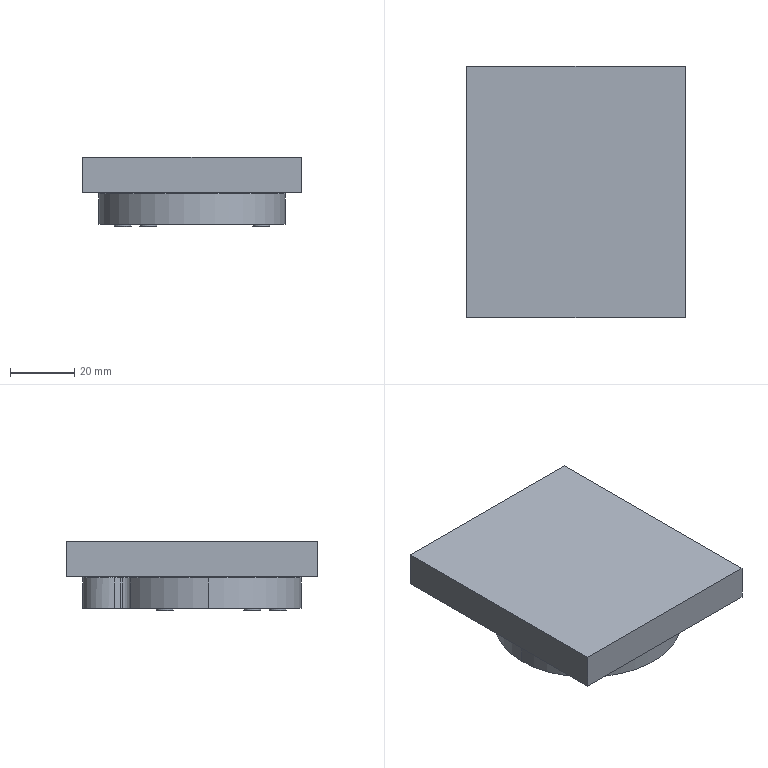NC program | NX | posted with a generic post | part box 68 x 78.27 x 21.8 mm
Lines 1 to 750 of 10371:
N10 G17 G21 G94 G90
(FLOOR_WALL_COPY , TOOL : D80)
N12 T19 M6
N14 G54
N16 G17 G0 G90 X72. Y0. S5000 M3
N18 G43 Z30. H19
N20 Z7.02
N22 G94 G1 Z4.02 F2000.
N24 X69.
N26 X-69.
N28 X-72.
N30 Z7.02
N32 G0 Z30.
N34 X72.
N36 Z6.04
N38 G1 Z3.04
N40 X69.
N42 X-69.
N44 X-72.
N46 Z6.04
N48 G0 Z30.
N50 X72.
N52 Z5.06
N54 G1 Z2.06
N56 X69.
N58 X-69.
N60 X-72.
N62 Z5.06
N64 G0 Z30.
N66 X72.
N68 Z4.08
N70 G1 Z1.08
N72 X69.
N74 X-69.
N76 X-72.
N78 Z4.08
N80 G0 Z30.
N82 X72.
N84 Z3.1
N86 G1 Z0.1
N88 X69.
N90 X-69.
N92 X-72.
N94 Z3.1
N96 G0 Z30.
(FLOOR_WALL_COPY_1 , TOOL : D80)
N98 X72.
N100 Z3.
N102 G1 Z0. F1200.
N104 X69.
N106 X-69.
N108 X-72.
N110 Z3.
N112 G0 Z30.
N114 M5
(CAVITY_MILL_COPY , TOOL : D10)
N116 T15 M6
N118 G54
N120 G17 G0 G90 X-35.997 Y-1.276 S9500 M3
N122 G43 Z30. H15
N124 Z0.8
N126 G94 G1 Z-0.7 F1000.
N128 X-29.997 Y2.188
N130 G3 X-29.497 Y3.054 R1.
N132 G1 Y11.775 F3500.
N134 G2 X-6.023 Y28.327 R34.
N136 G1 X-5.915 Y28.805
N138 G2 X-4.175 Y32.989 R13.25
N140 X-2.726 Y34.632 R7.
N142 G1 X16.962
N144 G2 X19.933 Y22.964 R13.25
N146 G1 X19.825 Y22.487
N148 G2 X30.345 Y10.202 R34.
N150 X29.497 Y4.339 R8.95
N152 G1 Y-22.045
N154 G2 X15.336 Y-35.479 R34.
N156 X9.474 Y-34.632 R8.95
N158 G1 X-16.909
N160 G2 X-30.345 Y-20.471 R34.
N162 X-29.497 Y-14.608 R8.95
N164 G1 Y3.054
N166 X-23.497
N168 Y10.094
N170 G2 X-4.96 Y22.422 R28.
N172 G3 X-0.17 Y27.005 R6.
N174 G1 X-0.062 Y27.483
N176 G2 X0.3 Y28.632 R7.25
N178 G1 X13.719
N180 G2 X14.081 Y24.287 R7.25
N182 G1 X13.973 Y23.809
N184 G3 X16.327 Y17.612 R6.
N186 G2 X17.706 Y16.556 R28.
N188 G3 X23.497 Y-0.26 R8.95
N190 G1 X23.237 Y0.912
N192 G2 X13.995 Y6.803 R7.75
N194 X23.237 Y0.912 R-7.75
N196 G1 X23.497 Y-0.26
N198 Y-20.363
N200 G2 X21.691 Y-22.841 R28.
N202 G3 X4.875 Y-28.632 R8.95
N204 G1 X6.047 Y-28.372
N206 G2 X11.938 Y-19.13 R7.75
N208 X6.047 Y-28.372 R-7.75
N210 G1 X4.875 Y-28.632
N212 X-15.228
N214 G2 X-17.706 Y-26.825 R28.
N216 G3 X-23.497 Y-10.01 R8.95
N218 G1 X-23.237 Y-11.182
N220 G2 X-13.995 Y-17.073 R7.75
N222 X-23.237 Y-11.182 R-7.75
N224 G1 X-23.497 Y-10.01
N226 Y3.054
N228 X-17.497
N230 Y8.202
N232 G2 X-3.897 Y16.517 R22.
N234 G3 X4.539 Y22.632 R12.
N236 G1 X7.826
N238 G3 X9.207 Y16.897 R12.
N240 X17.497 Y-5.908 R14.95
N242 G1 Y-12.26
N244 G3 X-0.773 Y-22.632 R14.95
N246 G1 X-7.125
N248 G3 X-17.497 Y-4.362 R14.95
N250 G1 Y3.054
N252 X-11.497
N254 Y5.993
N256 G2 X-2.834 Y10.612 R16.
N258 G3 X0.86 Y11.696 R18.
N260 X7.183 Y-6.758 R20.95
N262 X-1.623 Y-12.318 R20.95
N264 X-11.497 Y-0.375 R20.95
N266 G1 Y3.054
N268 X-5.497
N270 Y3.219
N272 G2 X-4.936 Y3.562 R10.
N274 G3 X-4.656 Y2.239 R26.95
N276 X-5.497 Y2.89 R26.95
N278 G1 Y3.054
N280 G3 X-5.997 Y3.92 R1.
N282 G1 Z0.8
N284 G0 Z30.
N286 X-5.507 Y3.356
N288 Z0.8
N290 G1 X-6.017 Y2.78 Z0.76 F1000.
N292 X-7.26 Y1.64 Z0.671
N294 X-8.069 Y0.652 Z0.604
N296 X-8.745 Y-0.431 Z0.537
N298 X-9.057 Y-1.137 Z0.497
N300 X-8.128 Y-1.796 Z0.437
N302 X-6.168 Y-3.554 Z0.299
N304 X-4.436 Y-5.536 Z0.161
N306 X-2.958 Y-7.715 Z0.023
N308 X-1.755 Y-10.057 Z-0.115
N310 X-1.353 Y-11.122 Z-0.174
N312 X-0.532 Y-10.333 Z-0.234
N314 X1.168 Y-9.006 Z-0.347
N316 X2.992 Y-7.854 Z-0.46
N318 X4.922 Y-6.89 Z-0.573
N320 X5.988 Y-6.488 Z-0.633
N322 X5.199 Y-5.667 Z-0.692
N324 X3.436 Y-3.324 Z-0.846
N326 X2.006 Y-0.764 Z-1.
N328 X0.936 Y1.966 Z-1.153
N330 X0.244 Y4.816 Z-1.307
N332 X0.111 Y5.947 Z-1.367
N334 X-0.683 Y5.774 Z-1.409
N336 X-2.29 Y5.552 Z-1.494
N338 X-3.528 Y5.21 Z-1.562
N340 X-4.272 Y4.893 Z-1.604
N342 X-4.805 Y4.149 Z-1.652
N344 X-5.411 Y3.464 Z-1.7
N346 G2 X-6.691 Y2.161 R17.6 F3500.
N348 G3 X-9.057 Y-1.137 R9.9
N350 G2 X-1.353 Y-11.122 R21.6
N352 X5.988 Y-6.488 R21.6
N354 X0.111 Y5.947 R21.6
N356 X-1.489 Y5.663 R21.1
N358 G3 X-4.272 Y4.893 R10.9
N360 G2 X-5.411 Y3.464 R17.6
N362 G1 X-9.903 Y7.442
N364 G2 X-10.747 Y6.583 R11.6
N366 G3 X-15.874 Y-4.222 R15.9
N368 G2 X-6.002 Y-19.859 R15.6
N370 G3 X-0.912 Y-21.009 R15.9
N372 G2 X14.724 Y-11.136 R15.6
N374 G3 X15.874 Y-6.047 R15.9
N376 G2 X6.074 Y10.341 R15.6
N378 X3.547 Y13.707 R16.1
N380 X-2.308 Y11.607 R15.1
N382 G3 X-8.444 Y9.504 R16.9
N384 G2 X-9.903 Y7.442 R11.6
N386 G1 X-14.395 Y11.42
N388 G2 X-14.802 Y11.005 R5.6
N390 G3 X-21.529 Y-9.149 R21.9
N392 G2 X-11.962 Y-18.733 R9.6
N394 X-12.88 Y-22.847 R9.6
N396 G3 X4.014 Y-26.664 R21.9
N398 G2 X17.712 Y-18.015 R9.6
N400 G3 X21.529 Y-1.121 R21.9
N402 G2 X12.881 Y12.577 R9.6
N404 G3 X12.029 Y13.166 R21.9
N406 G2 X7.724 Y23.832 R10.1
N408 G1 X8.131 Y25.631
N410 G3 X7.263 Y27.007 R1.15
N412 X5.888 Y26.138 R1.15
N414 G1 X5.578 Y24.769
N416 G2 X2.967 Y21.183 R5.6
N418 X-3.128 Y17.551 R9.1
N420 G3 X-13.209 Y13.572 R22.9
N422 G2 X-14.395 Y11.42 R5.6
N424 G3 X-14.595 Y10.44 R1.
N426 G1 Z-0.2
N428 G0 Z2.3
N430 X-5.507 Y3.356
N432 Z-0.2
N434 G1 X-6.017 Y2.78 Z-0.24 F1000.
N436 X-7.26 Y1.64 Z-0.329
N438 X-8.069 Y0.652 Z-0.396
N440 X-8.745 Y-0.431 Z-0.463
N442 X-9.057 Y-1.137 Z-0.503
N444 X-8.128 Y-1.796 Z-0.563
N446 X-6.168 Y-3.554 Z-0.701
N448 X-4.436 Y-5.536 Z-0.839
N450 X-2.958 Y-7.715 Z-0.977
N452 X-1.755 Y-10.057 Z-1.115
N454 X-1.353 Y-11.122 Z-1.174
N456 X-0.532 Y-10.333 Z-1.234
N458 X1.168 Y-9.006 Z-1.347
N460 X2.992 Y-7.854 Z-1.46
N462 X4.922 Y-6.89 Z-1.573
N464 X5.988 Y-6.488 Z-1.633
N466 X5.199 Y-5.667 Z-1.692
N468 X3.436 Y-3.324 Z-1.846
N470 X2.006 Y-0.764 Z-2.
N472 X0.936 Y1.966 Z-2.153
N474 X0.244 Y4.816 Z-2.307
N476 X0.111 Y5.947 Z-2.367
N478 X-0.683 Y5.774 Z-2.409
N480 X-2.29 Y5.552 Z-2.494
N482 X-3.528 Y5.21 Z-2.562
N484 X-4.272 Y4.893 Z-2.604
N486 X-4.805 Y4.149 Z-2.652
N488 X-5.411 Y3.464 Z-2.7
N490 G2 X-6.691 Y2.161 R17.6 F3500.
N492 G3 X-9.057 Y-1.137 R9.9
N494 G2 X-1.353 Y-11.122 R21.6
N496 X5.988 Y-6.488 R21.6
N498 X0.111 Y5.947 R21.6
N500 X-1.489 Y5.663 R21.1
N502 G3 X-4.272 Y4.893 R10.9
N504 G2 X-5.411 Y3.464 R17.6
N506 G1 X-9.903 Y7.442
N508 G2 X-10.747 Y6.583 R11.6
N510 G3 X-15.874 Y-4.222 R15.9
N512 G2 X-6.002 Y-19.859 R15.6
N514 G3 X-0.912 Y-21.009 R15.9
N516 G2 X14.724 Y-11.136 R15.6
N518 G3 X15.874 Y-6.047 R15.9
N520 G2 X6.074 Y10.341 R15.6
N522 X3.547 Y13.707 R16.1
N524 X-2.308 Y11.607 R15.1
N526 G3 X-8.444 Y9.504 R16.9
N528 G2 X-9.903 Y7.442 R11.6
N530 G1 X-14.395 Y11.42
N532 G2 X-14.802 Y11.005 R5.6
N534 G3 X-21.529 Y-9.149 R21.9
N536 G2 X-11.962 Y-18.733 R9.6
N538 X-12.88 Y-22.847 R9.6
N540 G3 X4.014 Y-26.664 R21.9
N542 G2 X17.712 Y-18.015 R9.6
N544 G3 X21.529 Y-1.121 R21.9
N546 G2 X12.881 Y12.577 R9.6
N548 G3 X12.029 Y13.166 R21.9
N550 G2 X7.724 Y23.832 R10.1
N552 G1 X8.131 Y25.631
N554 G3 X7.263 Y27.007 R1.15
N556 X5.888 Y26.138 R1.15
N558 G1 X5.578 Y24.769
N560 G2 X2.967 Y21.183 R5.6
N562 X-3.128 Y17.551 R9.1
N564 G3 X-13.209 Y13.572 R22.9
N566 G2 X-14.395 Y11.42 R5.6
N568 G3 X-14.595 Y10.44 R1.
N570 G1 Z-1.2
N572 G0 Z1.3
N574 X-5.507 Y3.356
N576 Z-1.2
N578 G1 X-6.017 Y2.78 Z-1.24 F1000.
N580 X-7.26 Y1.64 Z-1.329
N582 X-8.069 Y0.652 Z-1.396
N584 X-8.745 Y-0.431 Z-1.463
N586 X-9.057 Y-1.137 Z-1.503
N588 X-8.128 Y-1.796 Z-1.563
N590 X-6.168 Y-3.554 Z-1.701
N592 X-4.436 Y-5.536 Z-1.839
N594 X-2.958 Y-7.715 Z-1.977
N596 X-1.755 Y-10.057 Z-2.115
N598 X-1.353 Y-11.122 Z-2.174
N600 X-0.532 Y-10.333 Z-2.234
N602 X1.168 Y-9.006 Z-2.347
N604 X2.992 Y-7.854 Z-2.46
N606 X4.922 Y-6.89 Z-2.573
N608 X5.988 Y-6.488 Z-2.633
N610 X5.199 Y-5.667 Z-2.692
N612 X3.436 Y-3.324 Z-2.846
N614 X2.006 Y-0.764 Z-3.
N616 X0.936 Y1.966 Z-3.153
N618 X0.244 Y4.816 Z-3.307
N620 X0.111 Y5.947 Z-3.367
N622 X-0.683 Y5.774 Z-3.409
N624 X-2.29 Y5.552 Z-3.494
N626 X-3.528 Y5.21 Z-3.562
N628 X-4.272 Y4.893 Z-3.604
N630 X-4.805 Y4.149 Z-3.652
N632 X-5.411 Y3.464 Z-3.7
N634 G2 X-6.691 Y2.161 R17.6 F3500.
N636 G3 X-9.057 Y-1.137 R9.9
N638 G2 X-1.353 Y-11.122 R21.6
N640 X5.988 Y-6.488 R21.6
N642 X0.111 Y5.947 R21.6
N644 X-1.489 Y5.663 R21.1
N646 G3 X-4.272 Y4.893 R10.9
N648 G2 X-5.411 Y3.464 R17.6
N650 G1 X-9.903 Y7.442
N652 G2 X-10.747 Y6.583 R11.6
N654 G3 X-15.874 Y-4.222 R15.9
N656 G2 X-6.002 Y-19.859 R15.6
N658 G3 X-0.912 Y-21.009 R15.9
N660 G2 X14.724 Y-11.136 R15.6
N662 G3 X15.874 Y-6.047 R15.9
N664 G2 X6.074 Y10.341 R15.6
N666 X3.547 Y13.707 R16.1
N668 X-2.308 Y11.607 R15.1
N670 G3 X-8.444 Y9.504 R16.9
N672 G2 X-9.903 Y7.442 R11.6
N674 G1 X-14.395 Y11.42
N676 G2 X-14.802 Y11.005 R5.6
N678 G3 X-21.529 Y-9.149 R21.9
N680 G2 X-11.962 Y-18.733 R9.6
N682 X-12.88 Y-22.847 R9.6
N684 G3 X4.014 Y-26.664 R21.9
N686 G2 X17.712 Y-18.015 R9.6
N688 G3 X21.529 Y-1.121 R21.9
N690 G2 X12.881 Y12.577 R9.6
N692 G3 X12.029 Y13.166 R21.9
N694 G2 X7.724 Y23.832 R10.1
N696 G1 X8.131 Y25.631
N698 G3 X7.263 Y27.007 R1.15
N700 X5.888 Y26.138 R1.15
N702 G1 X5.578 Y24.769
N704 G2 X2.967 Y21.183 R5.6
N706 X-3.128 Y17.551 R9.1
N708 G3 X-13.209 Y13.572 R22.9
N710 G2 X-14.395 Y11.42 R5.6
N712 G3 X-14.595 Y10.44 R1.
N714 G1 Z-2.2
N716 G0 Z0.3
N718 X-5.507 Y3.356
N720 Z-2.2
N722 G1 X-6.017 Y2.78 Z-2.24 F1000.
N724 X-7.26 Y1.64 Z-2.329
N726 X-8.069 Y0.652 Z-2.396
N728 X-8.745 Y-0.431 Z-2.463
N730 X-9.057 Y-1.137 Z-2.503
N732 X-8.128 Y-1.796 Z-2.563
N734 X-6.168 Y-3.554 Z-2.701
N736 X-4.436 Y-5.536 Z-2.839
N738 X-2.958 Y-7.715 Z-2.977
N740 X-1.755 Y-10.057 Z-3.115
N742 X-1.353 Y-11.122 Z-3.174
N744 X-0.532 Y-10.333 Z-3.234
N746 X1.168 Y-9.006 Z-3.347
N748 X2.992 Y-7.854 Z-3.46
N750 X4.922 Y-6.89 Z-3.573
N752 X5.988 Y-6.488 Z-3.633
N754 X5.199 Y-5.667 Z-3.692
N756 X3.436 Y-3.324 Z-3.846
N758 X2.006 Y-0.764 Z-4.
N760 X0.936 Y1.966 Z-4.153
N762 X0.244 Y4.816 Z-4.307
N764 X0.111 Y5.947 Z-4.367
N766 X-0.683 Y5.774 Z-4.409
N768 X-2.29 Y5.552 Z-4.494
N770 X-3.528 Y5.21 Z-4.562
N772 X-4.272 Y4.893 Z-4.604
N774 X-4.805 Y4.149 Z-4.652
N776 X-5.411 Y3.464 Z-4.7
N778 G2 X-6.691 Y2.161 R17.6 F3500.
N780 G3 X-9.057 Y-1.137 R9.9
N782 G2 X-1.353 Y-11.122 R21.6
N784 X5.988 Y-6.488 R21.6
N786 X0.111 Y5.947 R21.6
N788 X-1.489 Y5.663 R21.1
N790 G3 X-4.272 Y4.893 R10.9
N792 G2 X-5.411 Y3.464 R17.6
N794 G1 X-9.903 Y7.442
N796 G2 X-10.747 Y6.583 R11.6
N798 G3 X-15.874 Y-4.222 R15.9
N800 G2 X-6.002 Y-19.859 R15.6
N802 G3 X-0.912 Y-21.009 R15.9
N804 G2 X14.724 Y-11.136 R15.6
N806 G3 X15.874 Y-6.047 R15.9
N808 G2 X6.074 Y10.341 R15.6
N810 X3.547 Y13.707 R16.1
N812 X-2.308 Y11.607 R15.1
N814 G3 X-8.444 Y9.504 R16.9
N816 G2 X-9.903 Y7.442 R11.6
N818 G1 X-14.395 Y11.42
N820 G2 X-14.802 Y11.005 R5.6
N822 G3 X-21.529 Y-9.149 R21.9
N824 G2 X-11.962 Y-18.733 R9.6
N826 X-12.88 Y-22.847 R9.601
N828 G3 X4.014 Y-26.663 R21.9
N830 G2 X17.712 Y-18.015 R9.6
N832 G3 X21.529 Y-1.121 R21.9
N834 G2 X12.881 Y12.577 R9.6
N836 G3 X12.029 Y13.166 R21.9
N838 G2 X7.724 Y23.832 R10.1
N840 G1 X8.131 Y25.631
N842 G3 X7.263 Y27.007 R1.15
N844 X5.888 Y26.138 R1.15
N846 G1 X5.578 Y24.769
N848 G2 X2.967 Y21.183 R5.6
N850 X-3.128 Y17.551 R9.1
N852 G3 X-13.209 Y13.572 R22.9
N854 G2 X-14.395 Y11.42 R5.6
N856 G3 X-14.595 Y10.44 R1.
N858 G1 Z-3.2
N860 G0 Z-0.7
N862 X-5.507 Y3.356
N864 Z-3.2
N866 G1 X-6.017 Y2.78 Z-3.24 F1000.
N868 X-7.26 Y1.64 Z-3.329
N870 X-8.069 Y0.652 Z-3.396
N872 X-8.745 Y-0.431 Z-3.463
N874 X-9.057 Y-1.137 Z-3.503
N876 X-8.128 Y-1.796 Z-3.563
N878 X-6.168 Y-3.554 Z-3.701
N880 X-4.436 Y-5.536 Z-3.839
N882 X-2.958 Y-7.715 Z-3.977
N884 X-1.755 Y-10.057 Z-4.115
N886 X-1.353 Y-11.122 Z-4.174
N888 X-0.532 Y-10.333 Z-4.234
N890 X1.168 Y-9.006 Z-4.347
N892 X2.992 Y-7.854 Z-4.46
N894 X4.922 Y-6.89 Z-4.573
N896 X5.988 Y-6.488 Z-4.633
N898 X5.199 Y-5.667 Z-4.692
N900 X3.436 Y-3.324 Z-4.846
N902 X2.006 Y-0.764 Z-5.
N904 X0.936 Y1.966 Z-5.153
N906 X0.244 Y4.816 Z-5.307
N908 X0.111 Y5.947 Z-5.367
N910 X-0.683 Y5.774 Z-5.409
N912 X-2.29 Y5.552 Z-5.494
N914 X-3.528 Y5.21 Z-5.562
N916 X-4.272 Y4.893 Z-5.604
N918 X-4.805 Y4.149 Z-5.652
N920 X-5.411 Y3.464 Z-5.7
N922 G2 X-6.691 Y2.161 R17.6 F3500.
N924 G3 X-9.057 Y-1.137 R9.9
N926 G2 X-1.353 Y-11.122 R21.6
N928 X5.988 Y-6.488 R21.6
N930 X0.111 Y5.947 R21.6
N932 X-1.489 Y5.663 R21.1
N934 G3 X-4.272 Y4.893 R10.9
N936 G2 X-5.411 Y3.464 R17.6
N938 G1 X-9.903 Y7.442
N940 G2 X-10.747 Y6.583 R11.6
N942 G3 X-15.874 Y-4.222 R15.9
N944 G2 X-6.002 Y-19.859 R15.6
N946 G3 X-0.912 Y-21.009 R15.9
N948 G2 X14.724 Y-11.136 R15.6
N950 G3 X15.874 Y-6.047 R15.9
N952 G2 X6.074 Y10.341 R15.6
N954 X3.547 Y13.707 R16.1
N956 X-2.308 Y11.607 R15.1
N958 G3 X-8.444 Y9.504 R16.9
N960 G2 X-9.903 Y7.442 R11.6
N962 G1 X-14.395 Y11.42
N964 G2 X-14.802 Y11.005 R5.6
N966 G3 X-21.529 Y-9.149 R21.9
N968 G2 X-11.962 Y-18.733 R9.6
N970 X-12.88 Y-22.847 R9.601
N972 G3 X4.014 Y-26.663 R21.9
N974 G2 X17.712 Y-18.015 R9.6
N976 G3 X21.528 Y-1.121 R21.9
N978 G2 X12.881 Y12.577 R9.6
N980 G3 X12.029 Y13.166 R21.9
N982 G2 X7.724 Y23.832 R10.1
N984 G1 X8.131 Y25.631
N986 G3 X7.263 Y27.007 R1.15
N988 X5.888 Y26.138 R1.15
N990 G1 X5.578 Y24.769
N992 G2 X2.967 Y21.183 R5.6
N994 X-3.128 Y17.551 R9.1
N996 G3 X-13.209 Y13.572 R22.9
N998 G2 X-14.395 Y11.42 R5.6
N1000 G3 X-14.595 Y10.44 R1.
N1002 G1 Z-4.2
N1004 G0 Z-1.7
N1006 X-5.507 Y3.356
N1008 Z-4.2
N1010 G1 X-6.017 Y2.78 Z-4.24 F1000.
N1012 X-7.26 Y1.64 Z-4.329
N1014 X-8.069 Y0.652 Z-4.396
N1016 X-8.745 Y-0.431 Z-4.463
N1018 X-9.057 Y-1.137 Z-4.503
N1020 X-8.128 Y-1.796 Z-4.563
N1022 X-6.168 Y-3.554 Z-4.701
N1024 X-4.436 Y-5.536 Z-4.839
N1026 X-2.958 Y-7.715 Z-4.977
N1028 X-1.755 Y-10.057 Z-5.115
N1030 X-1.353 Y-11.122 Z-5.174
N1032 X-0.532 Y-10.333 Z-5.234
N1034 X1.168 Y-9.006 Z-5.347
N1036 X2.992 Y-7.854 Z-5.46
N1038 X4.922 Y-6.89 Z-5.573
N1040 X5.988 Y-6.488 Z-5.633
N1042 X5.199 Y-5.667 Z-5.692
N1044 X3.436 Y-3.324 Z-5.846
N1046 X2.006 Y-0.764 Z-6.
N1048 X0.936 Y1.966 Z-6.153
N1050 X0.244 Y4.816 Z-6.307
N1052 X0.111 Y5.947 Z-6.367
N1054 X-0.683 Y5.774 Z-6.409
N1056 X-2.29 Y5.552 Z-6.494
N1058 X-3.528 Y5.21 Z-6.562
N1060 X-4.272 Y4.893 Z-6.604
N1062 X-4.805 Y4.149 Z-6.652
N1064 X-5.411 Y3.464 Z-6.7
N1066 G2 X-6.691 Y2.161 R17.6 F3500.
N1068 G3 X-9.057 Y-1.137 R9.9
N1070 G2 X-1.353 Y-11.122 R21.6
N1072 X5.988 Y-6.488 R21.6
N1074 X0.111 Y5.947 R21.6
N1076 X-1.489 Y5.663 R21.1
N1078 G3 X-4.272 Y4.893 R10.9
N1080 G2 X-5.411 Y3.464 R17.6
N1082 G1 X-9.903 Y7.442
N1084 G2 X-10.747 Y6.583 R11.6
N1086 G3 X-15.874 Y-4.222 R15.9
N1088 G2 X-6.002 Y-19.859 R15.6
N1090 G3 X-0.912 Y-21.009 R15.9
N1092 G2 X14.724 Y-11.136 R15.6
N1094 G3 X15.874 Y-6.047 R15.9
N1096 G2 X6.074 Y10.341 R15.6
N1098 X3.547 Y13.707 R16.1
N1100 X-2.308 Y11.607 R15.1
N1102 G3 X-8.444 Y9.504 R16.9
N1104 G2 X-9.903 Y7.442 R11.6
N1106 G1 X-14.395 Y11.42
N1108 G2 X-14.802 Y11.005 R5.6
N1110 G3 X-21.529 Y-9.149 R21.9
N1112 G2 X-11.962 Y-18.733 R9.6
N1114 X-12.88 Y-22.847 R9.601
N1116 G3 X4.014 Y-26.663 R21.9
N1118 G2 X17.712 Y-18.015 R9.6
N1120 G3 X21.528 Y-1.121 R21.9
N1122 G2 X12.881 Y12.577 R9.6
N1124 G3 X12.029 Y13.166 R21.9
N1126 G2 X7.724 Y23.832 R10.1
N1128 G1 X8.131 Y25.631
N1130 G3 X7.263 Y27.007 R1.15
N1132 X5.888 Y26.138 R1.15
N1134 G1 X5.578 Y24.769
N1136 G2 X2.967 Y21.183 R5.6
N1138 X-3.128 Y17.551 R9.1
N1140 G3 X-13.209 Y13.572 R22.9
N1142 G2 X-14.395 Y11.42 R5.6
N1144 G3 X-14.595 Y10.44 R1.
N1146 G1 Z-5.2
N1148 G0 Z-2.7
N1150 X-5.507 Y3.356
N1152 Z-5.2
N1154 G1 X-6.017 Y2.78 Z-5.24 F1000.
N1156 X-7.26 Y1.64 Z-5.329
N1158 X-8.069 Y0.652 Z-5.396
N1160 X-8.745 Y-0.431 Z-5.463
N1162 X-9.057 Y-1.137 Z-5.503
N1164 X-8.128 Y-1.796 Z-5.563
N1166 X-6.168 Y-3.554 Z-5.701
N1168 X-4.436 Y-5.536 Z-5.839
N1170 X-2.958 Y-7.715 Z-5.977
N1172 X-1.755 Y-10.057 Z-6.115
N1174 X-1.353 Y-11.122 Z-6.174
N1176 X-0.532 Y-10.333 Z-6.234
N1178 X1.168 Y-9.006 Z-6.347
N1180 X2.992 Y-7.854 Z-6.46
N1182 X4.922 Y-6.89 Z-6.573
N1184 X5.988 Y-6.488 Z-6.633
N1186 X5.199 Y-5.667 Z-6.692
N1188 X3.436 Y-3.324 Z-6.846
N1190 X2.006 Y-0.764 Z-7.
N1192 X0.936 Y1.966 Z-7.153
N1194 X0.244 Y4.816 Z-7.307
N1196 X0.111 Y5.947 Z-7.367
N1198 X-0.683 Y5.774 Z-7.409
N1200 X-2.29 Y5.552 Z-7.494
N1202 X-3.528 Y5.21 Z-7.562
N1204 X-4.272 Y4.893 Z-7.604
N1206 X-4.805 Y4.149 Z-7.652
N1208 X-5.411 Y3.464 Z-7.7
N1210 G2 X-6.691 Y2.161 R17.6 F3500.
N1212 G3 X-9.057 Y-1.137 R9.9
N1214 G2 X-1.353 Y-11.122 R21.6
N1216 X5.988 Y-6.488 R21.6
N1218 X0.111 Y5.947 R21.6
N1220 X-1.489 Y5.663 R21.1
N1222 G3 X-4.272 Y4.893 R10.9
N1224 G2 X-5.411 Y3.464 R17.6
N1226 G1 X-9.903 Y7.442
N1228 G2 X-10.747 Y6.583 R11.6
N1230 G3 X-15.874 Y-4.222 R15.9
N1232 G2 X-6.002 Y-19.859 R15.6
N1234 G3 X-0.912 Y-21.009 R15.9
N1236 G2 X14.724 Y-11.136 R15.6
N1238 G3 X15.874 Y-6.047 R15.9
N1240 G2 X6.074 Y10.341 R15.6
N1242 X3.547 Y13.707 R16.1
N1244 X-2.308 Y11.607 R15.1
N1246 G3 X-8.444 Y9.504 R16.9
N1248 G2 X-9.903 Y7.442 R11.6
N1250 G1 X-14.395 Y11.42
N1252 G2 X-14.802 Y11.005 R5.6
N1254 G3 X-21.529 Y-9.149 R21.9
N1256 G2 X-11.962 Y-18.733 R9.6
N1258 X-12.88 Y-22.847 R9.601
N1260 G3 X4.014 Y-26.663 R21.9
N1262 G2 X17.712 Y-18.015 R9.6
N1264 G3 X21.528 Y-1.121 R21.9
N1266 G2 X12.881 Y12.577 R9.6
N1268 G3 X12.029 Y13.166 R21.9
N1270 G2 X7.724 Y23.832 R10.1
N1272 G1 X8.131 Y25.631
N1274 G3 X5.878 Y26.094 R-1.15
N1276 G1 X5.75 Y25.528
N1278 X5.578 Y24.769
N1280 G2 X2.967 Y21.183 R5.6
N1282 X-3.128 Y17.551 R9.1
N1284 G3 X-13.209 Y13.572 R22.9
N1286 G2 X-14.395 Y11.42 R5.6
N1288 G3 X-14.595 Y10.44 R1.
N1290 G1 Z-6.2
N1292 G0 Z-3.7
N1294 X-5.507 Y3.356
N1296 Z-6.2
N1298 G1 X-6.017 Y2.78 Z-6.24 F1000.
N1300 X-7.26 Y1.64 Z-6.329
N1302 X-8.069 Y0.652 Z-6.396
N1304 X-8.745 Y-0.431 Z-6.463
N1306 X-9.057 Y-1.137 Z-6.503
N1308 X-8.128 Y-1.796 Z-6.563
N1310 X-6.168 Y-3.554 Z-6.701
N1312 X-4.436 Y-5.536 Z-6.839
N1314 X-2.958 Y-7.715 Z-6.977
N1316 X-1.755 Y-10.057 Z-7.115
N1318 X-1.353 Y-11.122 Z-7.174
N1320 X-0.532 Y-10.333 Z-7.234
N1322 X1.168 Y-9.006 Z-7.347
N1324 X2.992 Y-7.854 Z-7.46
N1326 X4.922 Y-6.89 Z-7.573
N1328 X5.988 Y-6.488 Z-7.633
N1330 X5.199 Y-5.667 Z-7.692
N1332 X3.436 Y-3.324 Z-7.846
N1334 X2.006 Y-0.764 Z-8.
N1336 X0.936 Y1.966 Z-8.153
N1338 X0.244 Y4.816 Z-8.307
N1340 X0.111 Y5.947 Z-8.367
N1342 X-0.683 Y5.774 Z-8.409
N1344 X-2.29 Y5.552 Z-8.494
N1346 X-3.528 Y5.21 Z-8.562
N1348 X-4.272 Y4.893 Z-8.604
N1350 X-4.805 Y4.149 Z-8.652
N1352 X-5.411 Y3.464 Z-8.7
N1354 G2 X-6.691 Y2.161 R17.6 F3500.
N1356 G3 X-9.057 Y-1.137 R9.9
N1358 G2 X-1.353 Y-11.122 R21.6
N1360 X5.988 Y-6.488 R21.6
N1362 X0.111 Y5.947 R21.6
N1364 X-1.489 Y5.663 R21.1
N1366 G3 X-4.272 Y4.893 R10.9
N1368 G2 X-5.411 Y3.464 R17.6
N1370 G1 X-9.903 Y7.442
N1372 G2 X-10.747 Y6.583 R11.6
N1374 G3 X-15.874 Y-4.222 R15.9
N1376 G2 X-6.002 Y-19.859 R15.6
N1378 G3 X-0.912 Y-21.009 R15.9
N1380 G2 X14.724 Y-11.136 R15.6
N1382 G3 X15.874 Y-6.047 R15.9
N1384 G2 X6.074 Y10.341 R15.6
N1386 X3.547 Y13.707 R16.1
N1388 X-2.308 Y11.607 R15.1
N1390 G3 X-8.444 Y9.504 R16.9
N1392 G2 X-9.903 Y7.442 R11.6
N1394 G1 X-14.395 Y11.42
N1396 G2 X-14.802 Y11.005 R5.6
N1398 G3 X-21.529 Y-9.149 R21.9
N1400 G2 X-11.962 Y-18.733 R9.6
N1402 X-12.88 Y-22.847 R9.601
N1404 G3 X4.014 Y-26.663 R21.9
N1406 G2 X17.712 Y-18.015 R9.6
N1408 G3 X21.528 Y-1.121 R21.9
N1410 G2 X12.881 Y12.577 R9.6
N1412 G3 X12.029 Y13.166 R21.9
N1414 G2 X7.724 Y23.832 R10.1
N1416 G1 X8.131 Y25.631
N1418 G3 X5.878 Y26.094 R-1.15
N1420 G1 X5.75 Y25.527
N1422 X5.578 Y24.769
N1424 G2 X2.967 Y21.183 R5.6
N1426 X-3.128 Y17.551 R9.1
N1428 G3 X-13.209 Y13.572 R22.9
N1430 G2 X-14.395 Y11.42 R5.6
N1432 G3 X-14.595 Y10.44 R1.
N1434 G1 Z-7.2
N1436 G0 Z-4.7
N1438 X-7.293 Y10.691
N1440 Z-7.2
N1442 G1 X5.456 Y19.116 Z-8.001 F1000.
N1444 X1.857 Y19.93 Z-8.194
N1446 X1.317 Y19.424 Z-8.233
N1448 X-0.438 Y18.326 Z-8.342
N1450 X-2.395 Y17.652 Z-8.45
N1452 X-3.128 Y17.551 Z-8.489
N1454 X-4.289 Y17.39 Z-8.55
N1456 X-6.465 Y16.865 Z-8.668
N1458 X-8.579 Y16.13 Z-8.785
N1460 X-10.611 Y15.192 Z-8.902
N1462 X-11.622 Y14.597 Z-8.964
N1464 X-8.569 Y9.847 Z-9.259
N1466 X-1.557 Y14.482 Z-9.7
N1468 X5.456 Y19.116 F3500.
N1470 X1.857 Y19.93
N1472 G2 X-3.128 Y17.551 R9.1
N1474 G3 X-11.622 Y14.597 R22.9
N1476 G1 X-8.569 Y9.847
N1478 X-1.557 Y14.482
N1480 G3 X-1.11 Y15.376 R1.
N1482 G1 Z-8.2
N1484 G0 Z30.
N1486 M5